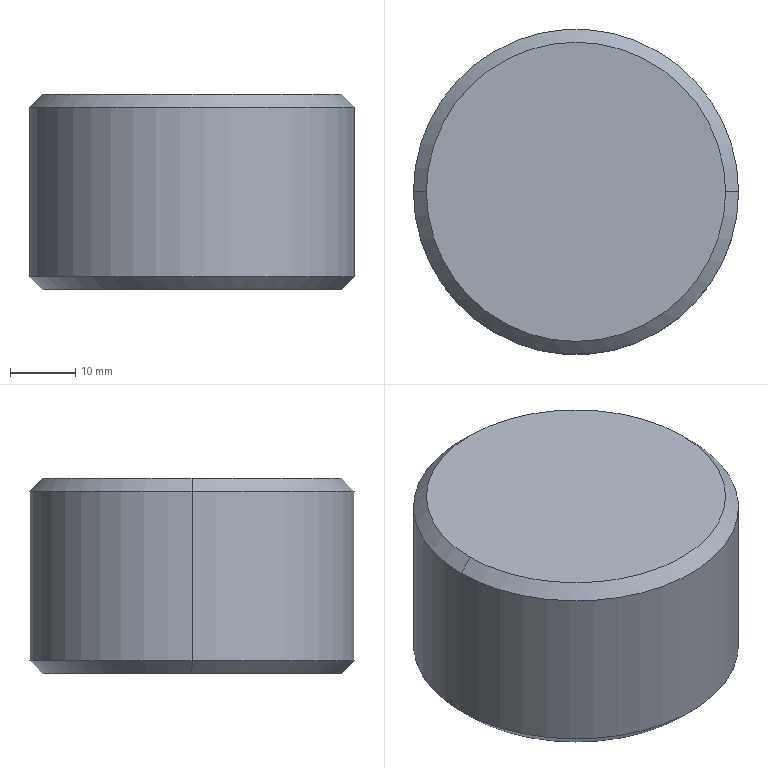Part | SolidWorks | features Chamfer 1, Extrusion 1 | 1 solid | 8 faces | box 50 x 50 x 30 mm | volume 58293 mm3 | cone 4 | cylinder 2 | plane 2 | commonest cylinder face diameters 50 x2
STEP:
#1=CARTESIAN_POINT('',(-23.,0.,0.));
#2=VERTEX_POINT('',#1);
#3=CARTESIAN_POINT('',(23.,0.,0.));
#4=VERTEX_POINT('',#3);
#5=CARTESIAN_POINT('',(0.,0.,0.));
#6=DIRECTION('',(0.,0.,-1.));
#7=DIRECTION('',(1.,0.,0.));
#8=AXIS2_PLACEMENT_3D('',#5,#6,#7);
#9=CIRCLE('',#8,23.);
#10=EDGE_CURVE('',#2,#4,#9,.T.);
#11=ORIENTED_EDGE('',*,*,#10,.F.);
#12=CARTESIAN_POINT('',(-25.,0.,2.));
#13=VERTEX_POINT('',#12);
#14=CARTESIAN_POINT('',(-25.,0.,2.));
#15=DIRECTION('',(-0.7071,0.,0.7071));
#16=VECTOR('',#15,1000.);
#17=LINE('',#14,#16);
#18=EDGE_CURVE('',#2,#13,#17,.T.);
#19=ORIENTED_EDGE('',*,*,#18,.T.);
#20=CARTESIAN_POINT('',(25.,0.,2.));
#21=VERTEX_POINT('',#20);
#22=CARTESIAN_POINT('',(0.,0.,2.));
#23=DIRECTION('',(0.,0.,1.));
#24=DIRECTION('',(1.,0.,0.));
#25=AXIS2_PLACEMENT_3D('',#22,#23,#24);
#26=CIRCLE('',#25,25.);
#27=EDGE_CURVE('',#21,#13,#26,.T.);
#28=ORIENTED_EDGE('',*,*,#27,.F.);
#29=CARTESIAN_POINT('',(25.,0.,2.));
#30=DIRECTION('',(0.7071,0.,0.7071));
#31=VECTOR('',#30,1000.);
#32=LINE('',#29,#31);
#33=EDGE_CURVE('',#4,#21,#32,.T.);
#34=ORIENTED_EDGE('',*,*,#33,.F.);
#35=EDGE_LOOP('',(#11,#19,#28,#34));
#36=FACE_OUTER_BOUND('',#35,.T.);
#37=CARTESIAN_POINT('',(0.,0.,2.));
#38=DIRECTION('',(0.,0.,1.));
#39=DIRECTION('',(1.,0.,0.));
#40=AXIS2_PLACEMENT_3D('',#37,#38,#39);
#41=CONICAL_SURFACE('',#40,25.,0.7854);
#42=ADVANCED_FACE('',(#36),#41,.T.);
#43=CARTESIAN_POINT('',(23.,0.,30.));
#44=VERTEX_POINT('',#43);
#45=CARTESIAN_POINT('',(-23.,0.,30.));
#46=VERTEX_POINT('',#45);
#47=CARTESIAN_POINT('',(0.,0.,30.));
#48=DIRECTION('',(0.,0.,1.));
#49=DIRECTION('',(1.,0.,0.));
#50=AXIS2_PLACEMENT_3D('',#47,#48,#49);
#51=CIRCLE('',#50,23.);
#52=EDGE_CURVE('',#44,#46,#51,.T.);
#53=ORIENTED_EDGE('',*,*,#52,.F.);
#54=CARTESIAN_POINT('',(25.,0.,28.));
#55=VERTEX_POINT('',#54);
#56=CARTESIAN_POINT('',(23.,0.,30.));
#57=DIRECTION('',(0.7071,0.,-0.7071));
#58=VECTOR('',#57,1000.);
#59=LINE('',#56,#58);
#60=EDGE_CURVE('',#44,#55,#59,.T.);
#61=ORIENTED_EDGE('',*,*,#60,.T.);
#62=CARTESIAN_POINT('',(-25.,0.,28.));
#63=VERTEX_POINT('',#62);
#64=CARTESIAN_POINT('',(0.,0.,28.));
#65=DIRECTION('',(0.,0.,-1.));
#66=DIRECTION('',(1.,0.,0.));
#67=AXIS2_PLACEMENT_3D('',#64,#65,#66);
#68=CIRCLE('',#67,25.);
#69=EDGE_CURVE('',#63,#55,#68,.T.);
#70=ORIENTED_EDGE('',*,*,#69,.F.);
#71=CARTESIAN_POINT('',(-23.,0.,30.));
#72=DIRECTION('',(-0.7071,0.,-0.7071));
#73=VECTOR('',#72,1000.);
#74=LINE('',#71,#73);
#75=EDGE_CURVE('',#46,#63,#74,.T.);
#76=ORIENTED_EDGE('',*,*,#75,.F.);
#77=EDGE_LOOP('',(#53,#61,#70,#76));
#78=FACE_OUTER_BOUND('',#77,.T.);
#79=CARTESIAN_POINT('',(0.,0.,30.));
#80=DIRECTION('',(0.,0.,-1.));
#81=DIRECTION('',(-1.,0.,0.));
#82=AXIS2_PLACEMENT_3D('',#79,#80,#81);
#83=CONICAL_SURFACE('',#82,23.,0.7854);
#84=ADVANCED_FACE('',(#78),#83,.T.);
#85=ORIENTED_EDGE('',*,*,#69,.T.);
#86=CARTESIAN_POINT('',(25.,0.,30.));
#87=DIRECTION('',(0.,0.,-1.));
#88=VECTOR('',#87,1000.);
#89=LINE('',#86,#88);
#90=EDGE_CURVE('',#55,#21,#89,.T.);
#91=ORIENTED_EDGE('',*,*,#90,.T.);
#92=ORIENTED_EDGE('',*,*,#27,.T.);
#93=CARTESIAN_POINT('',(-25.,0.,30.));
#94=DIRECTION('',(0.,0.,-1.));
#95=VECTOR('',#94,1000.);
#96=LINE('',#93,#95);
#97=EDGE_CURVE('',#63,#13,#96,.T.);
#98=ORIENTED_EDGE('',*,*,#97,.F.);
#99=EDGE_LOOP('',(#85,#91,#92,#98));
#100=FACE_OUTER_BOUND('',#99,.T.);
#101=CARTESIAN_POINT('',(0.,0.,30.));
#102=DIRECTION('',(0.,0.,-1.));
#103=DIRECTION('',(-1.,0.,0.));
#104=AXIS2_PLACEMENT_3D('',#101,#102,#103);
#105=CYLINDRICAL_SURFACE('',#104,25.);
#106=ADVANCED_FACE('',(#100),#105,.T.);
#107=ORIENTED_EDGE('',*,*,#90,.F.);
#108=CARTESIAN_POINT('',(0.,0.,28.));
#109=DIRECTION('',(0.,0.,-1.));
#110=DIRECTION('',(1.,0.,0.));
#111=AXIS2_PLACEMENT_3D('',#108,#109,#110);
#112=CIRCLE('',#111,25.);
#113=EDGE_CURVE('',#55,#63,#112,.T.);
#114=ORIENTED_EDGE('',*,*,#113,.T.);
#115=ORIENTED_EDGE('',*,*,#97,.T.);
#116=CARTESIAN_POINT('',(0.,0.,2.));
#117=DIRECTION('',(0.,0.,1.));
#118=DIRECTION('',(1.,0.,0.));
#119=AXIS2_PLACEMENT_3D('',#116,#117,#118);
#120=CIRCLE('',#119,25.);
#121=EDGE_CURVE('',#13,#21,#120,.T.);
#122=ORIENTED_EDGE('',*,*,#121,.T.);
#123=EDGE_LOOP('',(#107,#114,#115,#122));
#124=FACE_OUTER_BOUND('',#123,.T.);
#125=CARTESIAN_POINT('',(0.,0.,30.));
#126=DIRECTION('',(0.,0.,-1.));
#127=DIRECTION('',(-1.,0.,0.));
#128=AXIS2_PLACEMENT_3D('',#125,#126,#127);
#129=CYLINDRICAL_SURFACE('',#128,25.);
#130=ADVANCED_FACE('',(#124),#129,.T.);
#131=CARTESIAN_POINT('',(0.,0.,30.));
#132=DIRECTION('',(0.,0.,1.));
#133=DIRECTION('',(1.,0.,0.));
#134=AXIS2_PLACEMENT_3D('',#131,#132,#133);
#135=CIRCLE('',#134,23.);
#136=EDGE_CURVE('',#46,#44,#135,.T.);
#137=ORIENTED_EDGE('',*,*,#136,.T.);
#138=ORIENTED_EDGE('',*,*,#52,.T.);
#139=EDGE_LOOP('',(#137,#138));
#140=FACE_OUTER_BOUND('',#139,.T.);
#141=CARTESIAN_POINT('',(0.,0.,30.));
#142=DIRECTION('',(0.,0.,1.));
#143=DIRECTION('',(1.,0.,0.));
#144=AXIS2_PLACEMENT_3D('',#141,#142,#143);
#145=PLANE('',#144);
#146=ADVANCED_FACE('',(#140),#145,.T.);
#147=CARTESIAN_POINT('',(0.,0.,0.));
#148=DIRECTION('',(0.,0.,-1.));
#149=DIRECTION('',(1.,0.,0.));
#150=AXIS2_PLACEMENT_3D('',#147,#148,#149);
#151=CIRCLE('',#150,23.);
#152=EDGE_CURVE('',#4,#2,#151,.T.);
#153=ORIENTED_EDGE('',*,*,#152,.T.);
#154=ORIENTED_EDGE('',*,*,#10,.T.);
#155=EDGE_LOOP('',(#153,#154));
#156=FACE_OUTER_BOUND('',#155,.T.);
#157=CARTESIAN_POINT('',(0.,0.,0.));
#158=DIRECTION('',(0.,0.,1.));
#159=DIRECTION('',(1.,0.,0.));
#160=AXIS2_PLACEMENT_3D('',#157,#158,#159);
#161=PLANE('',#160);
#162=ADVANCED_FACE('',(#156),#161,.F.);
#163=ORIENTED_EDGE('',*,*,#60,.F.);
#164=ORIENTED_EDGE('',*,*,#136,.F.);
#165=ORIENTED_EDGE('',*,*,#75,.T.);
#166=ORIENTED_EDGE('',*,*,#113,.F.);
#167=EDGE_LOOP('',(#163,#164,#165,#166));
#168=FACE_OUTER_BOUND('',#167,.T.);
#169=CARTESIAN_POINT('',(0.,0.,30.));
#170=DIRECTION('',(0.,0.,-1.));
#171=DIRECTION('',(-1.,0.,0.));
#172=AXIS2_PLACEMENT_3D('',#169,#170,#171);
#173=CONICAL_SURFACE('',#172,23.,0.7854);
#174=ADVANCED_FACE('',(#168),#173,.T.);
#175=ORIENTED_EDGE('',*,*,#18,.F.);
#176=ORIENTED_EDGE('',*,*,#152,.F.);
#177=ORIENTED_EDGE('',*,*,#33,.T.);
#178=ORIENTED_EDGE('',*,*,#121,.F.);
#179=EDGE_LOOP('',(#175,#176,#177,#178));
#180=FACE_OUTER_BOUND('',#179,.T.);
#181=CARTESIAN_POINT('',(0.,0.,2.));
#182=DIRECTION('',(0.,0.,1.));
#183=DIRECTION('',(1.,0.,0.));
#184=AXIS2_PLACEMENT_3D('',#181,#182,#183);
#185=CONICAL_SURFACE('',#184,25.,0.7854);
#186=ADVANCED_FACE('',(#180),#185,.T.);
#187=CLOSED_SHELL('',(#42,#84,#106,#130,#146,#162,#174,#186));
#188=MANIFOLD_SOLID_BREP('',#187);
#189=CARTESIAN_POINT('',(0.,0.,0.));
#190=DIRECTION('',(0.,0.,1.));
#191=DIRECTION('',(1.,0.,0.));
#192=AXIS2_PLACEMENT_3D('',#189,#190,#191);
#193=(LENGTH_UNIT()NAMED_UNIT(*)SI_UNIT(.MILLI.,.METRE.));
#194=UNCERTAINTY_MEASURE_WITH_UNIT(LENGTH_MEASURE(0.00001),#193,'','');
#195=(NAMED_UNIT(*)PLANE_ANGLE_UNIT()SI_UNIT($,.RADIAN.));
#196=(NAMED_UNIT(*)SI_UNIT($,.STERADIAN.)SOLID_ANGLE_UNIT());
#197=(GEOMETRIC_REPRESENTATION_CONTEXT(3)GLOBAL_UNCERTAINTY_ASSIGNED_CONTEXT((#194))GLOBAL_UNIT_ASSIGNED_CONTEXT((#193,#195,#196))REPRESENTATION_CONTEXT('',''));
#198=ADVANCED_BREP_SHAPE_REPRESENTATION('',(#188,#192),#197);